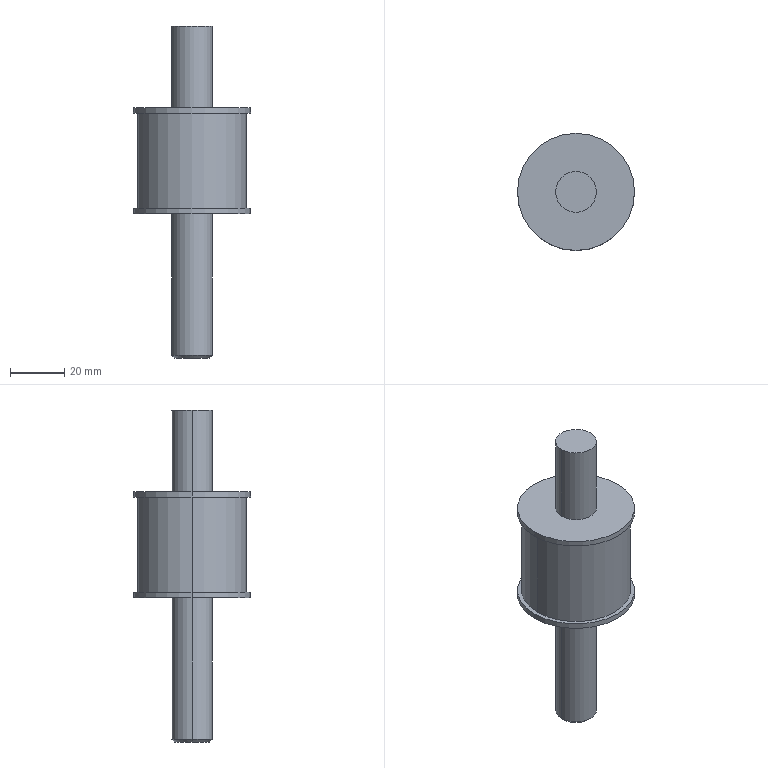Part | STEP file | Driving wheel | 1 solid | 18 faces | box 43 x 43 x 122 mm | volume 64436 mm3 | cylinder 10 | plane 6 | cone 2 | commonest cylinder face diameters 15 x4 43 x4 40 x2
STEP:
#1=CARTESIAN_POINT('',(0.,0.,0.));
#2=DIRECTION('',(0.,0.,1.));
#3=DIRECTION('',(1.,0.,0.));
#4=AXIS2_PLACEMENT_3D('',#1,#2,#3);
#5=CARTESIAN_POINT('',(-20.,0.,35.));
#6=VERTEX_POINT('',#5);
#7=CARTESIAN_POINT('',(20.,0.,35.));
#8=VERTEX_POINT('',#7);
#9=CARTESIAN_POINT('',(0.,0.,35.));
#10=DIRECTION('',(0.,0.,-1.));
#11=DIRECTION('',(-1.,0.,0.));
#12=AXIS2_PLACEMENT_3D('',#9,#10,#11);
#13=CIRCLE('',#12,20.);
#14=CARTESIAN_POINT('',(0.,0.,35.));
#15=DIRECTION('',(0.,0.,-1.));
#16=DIRECTION('',(-1.,0.,0.));
#17=AXIS2_PLACEMENT_3D('',#14,#15,#16);
#18=CYLINDRICAL_SURFACE('',#17,20.);
#19=CARTESIAN_POINT('',(0.,0.));
#20=DIRECTION('',(1.,0.));
#21=VECTOR('',#20,1.);
#22=LINE('',#19,#21);
#23=(GEOMETRIC_REPRESENTATION_CONTEXT(2)PARAMETRIC_REPRESENTATION_CONTEXT()REPRESENTATION_CONTEXT('',''));
#24=DEFINITIONAL_REPRESENTATION('',(#22),#23);
#25=PCURVE('',#18,#24);
#26=CARTESIAN_POINT('',(0.,0.,35.));
#27=DIRECTION('',(0.,0.,1.));
#28=DIRECTION('',(1.,0.,0.));
#29=AXIS2_PLACEMENT_3D('',#26,#27,#28);
#30=PLANE('',#29);
#31=CARTESIAN_POINT('',(-20.,0.));
#32=CARTESIAN_POINT('',(-20.,34.641));
#33=CARTESIAN_POINT('',(10.,17.321));
#34=CARTESIAN_POINT('',(40.,0.));
#35=CARTESIAN_POINT('',(10.,-17.321));
#36=CARTESIAN_POINT('',(-20.,-34.641));
#37=CARTESIAN_POINT('',(-20.,0.));
#38=(BOUNDED_CURVE()B_SPLINE_CURVE(2,(#31,#32,#33,#34,#35,#36,#37),.UNSPECIFIED.,.T.,.F.)B_SPLINE_CURVE_WITH_KNOTS((1,2,2,2,2,1),(-2.094,0.,2.094,4.189,6.283,8.378),.UNSPECIFIED.)CURVE()GEOMETRIC_REPRESENTATION_ITEM()RATIONAL_B_SPLINE_CURVE((1.,0.5,1.,0.5,1.,0.5,1.))REPRESENTATION_ITEM(''));
#39=(GEOMETRIC_REPRESENTATION_CONTEXT(2)PARAMETRIC_REPRESENTATION_CONTEXT()REPRESENTATION_CONTEXT('',''));
#40=DEFINITIONAL_REPRESENTATION('',(#38),#39);
#41=PCURVE('',#30,#40);
#42=SURFACE_CURVE('',#13,(#25,#41),.PCURVE_S1.);
#43=EDGE_CURVE('',#6,#8,#42,.T.);
#44=ORIENTED_EDGE('',*,*,#43,.T.);
#45=CARTESIAN_POINT('',(20.,0.,0.));
#46=VERTEX_POINT('',#45);
#47=CARTESIAN_POINT('',(20.,0.,35.));
#48=DIRECTION('',(0.,0.,-1.));
#49=VECTOR('',#48,1.);
#50=LINE('',#47,#49);
#51=CARTESIAN_POINT('',(3.142,0.));
#52=DIRECTION('',(0.,1.));
#53=VECTOR('',#52,1.);
#54=LINE('',#51,#53);
#55=(GEOMETRIC_REPRESENTATION_CONTEXT(2)PARAMETRIC_REPRESENTATION_CONTEXT()REPRESENTATION_CONTEXT('',''));
#56=DEFINITIONAL_REPRESENTATION('',(#54),#55);
#57=PCURVE('',#18,#56);
#58=CARTESIAN_POINT('',(0.,0.,35.));
#59=DIRECTION('',(0.,0.,-1.));
#60=DIRECTION('',(-1.,0.,0.));
#61=AXIS2_PLACEMENT_3D('',#58,#59,#60);
#62=CYLINDRICAL_SURFACE('',#61,20.);
#63=CARTESIAN_POINT('',(3.142,0.));
#64=DIRECTION('',(0.,1.));
#65=VECTOR('',#64,1.);
#66=LINE('',#63,#65);
#67=(GEOMETRIC_REPRESENTATION_CONTEXT(2)PARAMETRIC_REPRESENTATION_CONTEXT()REPRESENTATION_CONTEXT('',''));
#68=DEFINITIONAL_REPRESENTATION('',(#66),#67);
#69=PCURVE('',#62,#68);
#70=SURFACE_CURVE('',#50,(#57,#69),.PCURVE_S1.);
#71=EDGE_CURVE('',#8,#46,#70,.T.);
#72=ORIENTED_EDGE('',*,*,#71,.T.);
#73=CARTESIAN_POINT('',(-20.,0.,0.));
#74=VERTEX_POINT('',#73);
#75=CARTESIAN_POINT('',(0.,0.,0.));
#76=DIRECTION('',(0.,0.,1.));
#77=DIRECTION('',(-1.,0.,0.));
#78=AXIS2_PLACEMENT_3D('',#75,#76,#77);
#79=CIRCLE('',#78,20.);
#80=CARTESIAN_POINT('',(6.283,35.));
#81=DIRECTION('',(-1.,0.));
#82=VECTOR('',#81,1.);
#83=LINE('',#80,#82);
#84=(GEOMETRIC_REPRESENTATION_CONTEXT(2)PARAMETRIC_REPRESENTATION_CONTEXT()REPRESENTATION_CONTEXT('',''));
#85=DEFINITIONAL_REPRESENTATION('',(#83),#84);
#86=PCURVE('',#18,#85);
#87=CARTESIAN_POINT('',(0.,0.,0.));
#88=DIRECTION('',(0.,0.,-1.));
#89=DIRECTION('',(-1.,0.,0.));
#90=AXIS2_PLACEMENT_3D('',#87,#88,#89);
#91=PLANE('',#90);
#92=CARTESIAN_POINT('',(20.,0.));
#93=CARTESIAN_POINT('',(20.,-34.641));
#94=CARTESIAN_POINT('',(-10.,-17.321));
#95=CARTESIAN_POINT('',(-40.,0.));
#96=CARTESIAN_POINT('',(-10.,17.321));
#97=CARTESIAN_POINT('',(20.,34.641));
#98=CARTESIAN_POINT('',(20.,0.));
#99=(BOUNDED_CURVE()B_SPLINE_CURVE(2,(#92,#93,#94,#95,#96,#97,#98),.UNSPECIFIED.,.T.,.F.)B_SPLINE_CURVE_WITH_KNOTS((1,2,2,2,2,1),(-2.094,0.,2.094,4.189,6.283,8.378),.UNSPECIFIED.)CURVE()GEOMETRIC_REPRESENTATION_ITEM()RATIONAL_B_SPLINE_CURVE((1.,0.5,1.,0.5,1.,0.5,1.))REPRESENTATION_ITEM(''));
#100=(GEOMETRIC_REPRESENTATION_CONTEXT(2)PARAMETRIC_REPRESENTATION_CONTEXT()REPRESENTATION_CONTEXT('',''));
#101=DEFINITIONAL_REPRESENTATION('',(#99),#100);
#102=PCURVE('',#91,#101);
#103=SURFACE_CURVE('',#79,(#86,#102),.PCURVE_S1.);
#104=EDGE_CURVE('',#46,#74,#103,.T.);
#105=ORIENTED_EDGE('',*,*,#104,.T.);
#106=CARTESIAN_POINT('',(-20.,0.,35.));
#107=DIRECTION('',(0.,0.,-1.));
#108=VECTOR('',#107,1.);
#109=LINE('',#106,#108);
#110=CARTESIAN_POINT('',(0.,0.));
#111=DIRECTION('',(0.,1.));
#112=VECTOR('',#111,1.);
#113=LINE('',#110,#112);
#114=(GEOMETRIC_REPRESENTATION_CONTEXT(2)PARAMETRIC_REPRESENTATION_CONTEXT()REPRESENTATION_CONTEXT('',''));
#115=DEFINITIONAL_REPRESENTATION('',(#113),#114);
#116=PCURVE('',#18,#115);
#117=CARTESIAN_POINT('',(6.283,0.));
#118=DIRECTION('',(0.,1.));
#119=VECTOR('',#118,1.);
#120=LINE('',#117,#119);
#121=(GEOMETRIC_REPRESENTATION_CONTEXT(2)PARAMETRIC_REPRESENTATION_CONTEXT()REPRESENTATION_CONTEXT('',''));
#122=DEFINITIONAL_REPRESENTATION('',(#120),#121);
#123=PCURVE('',#62,#122);
#124=SURFACE_CURVE('',#109,(#116,#123),.PCURVE_S1.);
#125=EDGE_CURVE('',#6,#74,#124,.T.);
#126=ORIENTED_EDGE('',*,*,#125,.F.);
#127=EDGE_LOOP('',(#44,#72,#105,#126));
#128=FACE_BOUND('',#127,.T.);
#129=ADVANCED_FACE('',(#128),#18,.T.);
#130=CARTESIAN_POINT('',(21.5,0.,-2.));
#131=VERTEX_POINT('',#130);
#132=CARTESIAN_POINT('',(-21.5,0.,-2.));
#133=VERTEX_POINT('',#132);
#134=CARTESIAN_POINT('',(0.,0.,-2.));
#135=DIRECTION('',(0.,0.,1.));
#136=DIRECTION('',(1.,0.,0.));
#137=AXIS2_PLACEMENT_3D('',#134,#135,#136);
#138=CIRCLE('',#137,21.5);
#139=CARTESIAN_POINT('',(0.,0.,-2.));
#140=DIRECTION('',(0.,0.,1.));
#141=DIRECTION('',(1.,0.,0.));
#142=AXIS2_PLACEMENT_3D('',#139,#140,#141);
#143=CYLINDRICAL_SURFACE('',#142,21.5);
#144=CARTESIAN_POINT('',(0.,0.));
#145=DIRECTION('',(1.,0.));
#146=VECTOR('',#145,1.);
#147=LINE('',#144,#146);
#148=(GEOMETRIC_REPRESENTATION_CONTEXT(2)PARAMETRIC_REPRESENTATION_CONTEXT()REPRESENTATION_CONTEXT('',''));
#149=DEFINITIONAL_REPRESENTATION('',(#147),#148);
#150=PCURVE('',#143,#149);
#151=CARTESIAN_POINT('',(0.,0.,-2.));
#152=DIRECTION('',(0.,0.,-1.));
#153=DIRECTION('',(-1.,0.,0.));
#154=AXIS2_PLACEMENT_3D('',#151,#152,#153);
#155=PLANE('',#154);
#156=CARTESIAN_POINT('',(-21.5,0.));
#157=CARTESIAN_POINT('',(-21.5,37.239));
#158=CARTESIAN_POINT('',(10.75,18.62));
#159=CARTESIAN_POINT('',(43.,0.));
#160=CARTESIAN_POINT('',(10.75,-18.62));
#161=CARTESIAN_POINT('',(-21.5,-37.239));
#162=CARTESIAN_POINT('',(-21.5,0.));
#163=(BOUNDED_CURVE()B_SPLINE_CURVE(2,(#156,#157,#158,#159,#160,#161,#162),.UNSPECIFIED.,.T.,.F.)B_SPLINE_CURVE_WITH_KNOTS((1,2,2,2,2,1),(-2.094,0.,2.094,4.189,6.283,8.378),.UNSPECIFIED.)CURVE()GEOMETRIC_REPRESENTATION_ITEM()RATIONAL_B_SPLINE_CURVE((1.,0.5,1.,0.5,1.,0.5,1.))REPRESENTATION_ITEM(''));
#164=(GEOMETRIC_REPRESENTATION_CONTEXT(2)PARAMETRIC_REPRESENTATION_CONTEXT()REPRESENTATION_CONTEXT('',''));
#165=DEFINITIONAL_REPRESENTATION('',(#163),#164);
#166=PCURVE('',#155,#165);
#167=SURFACE_CURVE('',#138,(#150,#166),.PCURVE_S1.);
#168=EDGE_CURVE('',#131,#133,#167,.T.);
#169=ORIENTED_EDGE('',*,*,#168,.T.);
#170=CARTESIAN_POINT('',(-21.5,0.,0.));
#171=VERTEX_POINT('',#170);
#172=CARTESIAN_POINT('',(-21.5,0.,-2.));
#173=DIRECTION('',(0.,0.,1.));
#174=VECTOR('',#173,1.);
#175=LINE('',#172,#174);
#176=CARTESIAN_POINT('',(3.142,0.));
#177=DIRECTION('',(0.,1.));
#178=VECTOR('',#177,1.);
#179=LINE('',#176,#178);
#180=(GEOMETRIC_REPRESENTATION_CONTEXT(2)PARAMETRIC_REPRESENTATION_CONTEXT()REPRESENTATION_CONTEXT('',''));
#181=DEFINITIONAL_REPRESENTATION('',(#179),#180);
#182=PCURVE('',#143,#181);
#183=CARTESIAN_POINT('',(0.,0.,-2.));
#184=DIRECTION('',(0.,0.,1.));
#185=DIRECTION('',(1.,0.,0.));
#186=AXIS2_PLACEMENT_3D('',#183,#184,#185);
#187=CYLINDRICAL_SURFACE('',#186,21.5);
#188=CARTESIAN_POINT('',(3.142,0.));
#189=DIRECTION('',(0.,1.));
#190=VECTOR('',#189,1.);
#191=LINE('',#188,#190);
#192=(GEOMETRIC_REPRESENTATION_CONTEXT(2)PARAMETRIC_REPRESENTATION_CONTEXT()REPRESENTATION_CONTEXT('',''));
#193=DEFINITIONAL_REPRESENTATION('',(#191),#192);
#194=PCURVE('',#187,#193);
#195=SURFACE_CURVE('',#175,(#182,#194),.PCURVE_S1.);
#196=EDGE_CURVE('',#133,#171,#195,.T.);
#197=ORIENTED_EDGE('',*,*,#196,.T.);
#198=CARTESIAN_POINT('',(21.5,0.,0.));
#199=VERTEX_POINT('',#198);
#200=CARTESIAN_POINT('',(0.,0.,0.));
#201=DIRECTION('',(0.,0.,-1.));
#202=DIRECTION('',(1.,0.,0.));
#203=AXIS2_PLACEMENT_3D('',#200,#201,#202);
#204=CIRCLE('',#203,21.5);
#205=CARTESIAN_POINT('',(6.283,2.));
#206=DIRECTION('',(-1.,0.));
#207=VECTOR('',#206,1.);
#208=LINE('',#205,#207);
#209=(GEOMETRIC_REPRESENTATION_CONTEXT(2)PARAMETRIC_REPRESENTATION_CONTEXT()REPRESENTATION_CONTEXT('',''));
#210=DEFINITIONAL_REPRESENTATION('',(#208),#209);
#211=PCURVE('',#143,#210);
#212=CARTESIAN_POINT('',(0.,0.));
#213=DIRECTION('',(-1.,0.));
#214=AXIS2_PLACEMENT_2D('',#212,#213);
#215=CIRCLE('',#214,21.5);
#216=(GEOMETRIC_REPRESENTATION_CONTEXT(2)PARAMETRIC_REPRESENTATION_CONTEXT()REPRESENTATION_CONTEXT('',''));
#217=DEFINITIONAL_REPRESENTATION('',(#215),#216);
#218=PCURVE('',#91,#217);
#219=SURFACE_CURVE('',#204,(#211,#218),.PCURVE_S1.);
#220=EDGE_CURVE('',#171,#199,#219,.T.);
#221=ORIENTED_EDGE('',*,*,#220,.T.);
#222=CARTESIAN_POINT('',(21.5,0.,-2.));
#223=DIRECTION('',(0.,0.,1.));
#224=VECTOR('',#223,1.);
#225=LINE('',#222,#224);
#226=CARTESIAN_POINT('',(0.,0.));
#227=DIRECTION('',(0.,1.));
#228=VECTOR('',#227,1.);
#229=LINE('',#226,#228);
#230=(GEOMETRIC_REPRESENTATION_CONTEXT(2)PARAMETRIC_REPRESENTATION_CONTEXT()REPRESENTATION_CONTEXT('',''));
#231=DEFINITIONAL_REPRESENTATION('',(#229),#230);
#232=PCURVE('',#143,#231);
#233=CARTESIAN_POINT('',(6.283,0.));
#234=DIRECTION('',(0.,1.));
#235=VECTOR('',#234,1.);
#236=LINE('',#233,#235);
#237=(GEOMETRIC_REPRESENTATION_CONTEXT(2)PARAMETRIC_REPRESENTATION_CONTEXT()REPRESENTATION_CONTEXT('',''));
#238=DEFINITIONAL_REPRESENTATION('',(#236),#237);
#239=PCURVE('',#187,#238);
#240=SURFACE_CURVE('',#225,(#232,#239),.PCURVE_S1.);
#241=EDGE_CURVE('',#131,#199,#240,.T.);
#242=ORIENTED_EDGE('',*,*,#241,.F.);
#243=EDGE_LOOP('',(#169,#197,#221,#242));
#244=FACE_BOUND('',#243,.T.);
#245=ADVANCED_FACE('',(#244),#143,.T.);
#246=CARTESIAN_POINT('',(-21.5,0.,37.));
#247=VERTEX_POINT('',#246);
#248=CARTESIAN_POINT('',(21.5,0.,37.));
#249=VERTEX_POINT('',#248);
#250=CARTESIAN_POINT('',(0.,0.,37.));
#251=DIRECTION('',(0.,0.,-1.));
#252=DIRECTION('',(-1.,0.,0.));
#253=AXIS2_PLACEMENT_3D('',#250,#251,#252);
#254=CIRCLE('',#253,21.5);
#255=CARTESIAN_POINT('',(0.,0.,37.));
#256=DIRECTION('',(0.,0.,-1.));
#257=DIRECTION('',(-1.,0.,0.));
#258=AXIS2_PLACEMENT_3D('',#255,#256,#257);
#259=CYLINDRICAL_SURFACE('',#258,21.5);
#260=CARTESIAN_POINT('',(0.,0.));
#261=DIRECTION('',(1.,0.));
#262=VECTOR('',#261,1.);
#263=LINE('',#260,#262);
#264=(GEOMETRIC_REPRESENTATION_CONTEXT(2)PARAMETRIC_REPRESENTATION_CONTEXT()REPRESENTATION_CONTEXT('',''));
#265=DEFINITIONAL_REPRESENTATION('',(#263),#264);
#266=PCURVE('',#259,#265);
#267=CARTESIAN_POINT('',(0.,0.,37.));
#268=DIRECTION('',(0.,0.,1.));
#269=DIRECTION('',(1.,0.,0.));
#270=AXIS2_PLACEMENT_3D('',#267,#268,#269);
#271=PLANE('',#270);
#272=CARTESIAN_POINT('',(-21.5,0.));
#273=CARTESIAN_POINT('',(-21.5,37.239));
#274=CARTESIAN_POINT('',(10.75,18.62));
#275=CARTESIAN_POINT('',(43.,0.));
#276=CARTESIAN_POINT('',(10.75,-18.62));
#277=CARTESIAN_POINT('',(-21.5,-37.239));
#278=CARTESIAN_POINT('',(-21.5,0.));
#279=(BOUNDED_CURVE()B_SPLINE_CURVE(2,(#272,#273,#274,#275,#276,#277,#278),.UNSPECIFIED.,.T.,.F.)B_SPLINE_CURVE_WITH_KNOTS((1,2,2,2,2,1),(-2.094,0.,2.094,4.189,6.283,8.378),.UNSPECIFIED.)CURVE()GEOMETRIC_REPRESENTATION_ITEM()RATIONAL_B_SPLINE_CURVE((1.,0.5,1.,0.5,1.,0.5,1.))REPRESENTATION_ITEM(''));
#280=(GEOMETRIC_REPRESENTATION_CONTEXT(2)PARAMETRIC_REPRESENTATION_CONTEXT()REPRESENTATION_CONTEXT('',''));
#281=DEFINITIONAL_REPRESENTATION('',(#279),#280);
#282=PCURVE('',#271,#281);
#283=SURFACE_CURVE('',#254,(#266,#282),.PCURVE_S1.);
#284=EDGE_CURVE('',#247,#249,#283,.T.);
#285=ORIENTED_EDGE('',*,*,#284,.T.);
#286=CARTESIAN_POINT('',(21.5,0.,35.));
#287=VERTEX_POINT('',#286);
#288=CARTESIAN_POINT('',(21.5,0.,37.));
#289=DIRECTION('',(0.,0.,-1.));
#290=VECTOR('',#289,1.);
#291=LINE('',#288,#290);
#292=CARTESIAN_POINT('',(3.142,0.));
#293=DIRECTION('',(0.,1.));
#294=VECTOR('',#293,1.);
#295=LINE('',#292,#294);
#296=(GEOMETRIC_REPRESENTATION_CONTEXT(2)PARAMETRIC_REPRESENTATION_CONTEXT()REPRESENTATION_CONTEXT('',''));
#297=DEFINITIONAL_REPRESENTATION('',(#295),#296);
#298=PCURVE('',#259,#297);
#299=CARTESIAN_POINT('',(0.,0.,37.));
#300=DIRECTION('',(0.,0.,-1.));
#301=DIRECTION('',(-1.,0.,0.));
#302=AXIS2_PLACEMENT_3D('',#299,#300,#301);
#303=CYLINDRICAL_SURFACE('',#302,21.5);
#304=CARTESIAN_POINT('',(3.142,0.));
#305=DIRECTION('',(0.,1.));
#306=VECTOR('',#305,1.);
#307=LINE('',#304,#306);
#308=(GEOMETRIC_REPRESENTATION_CONTEXT(2)PARAMETRIC_REPRESENTATION_CONTEXT()REPRESENTATION_CONTEXT('',''));
#309=DEFINITIONAL_REPRESENTATION('',(#307),#308);
#310=PCURVE('',#303,#309);
#311=SURFACE_CURVE('',#291,(#298,#310),.PCURVE_S1.);
#312=EDGE_CURVE('',#249,#287,#311,.T.);
#313=ORIENTED_EDGE('',*,*,#312,.T.);
#314=CARTESIAN_POINT('',(-21.5,0.,35.));
#315=VERTEX_POINT('',#314);
#316=CARTESIAN_POINT('',(0.,0.,35.));
#317=DIRECTION('',(0.,0.,1.));
#318=DIRECTION('',(-1.,0.,0.));
#319=AXIS2_PLACEMENT_3D('',#316,#317,#318);
#320=CIRCLE('',#319,21.5);
#321=CARTESIAN_POINT('',(6.283,2.));
#322=DIRECTION('',(-1.,0.));
#323=VECTOR('',#322,1.);
#324=LINE('',#321,#323);
#325=(GEOMETRIC_REPRESENTATION_CONTEXT(2)PARAMETRIC_REPRESENTATION_CONTEXT()REPRESENTATION_CONTEXT('',''));
#326=DEFINITIONAL_REPRESENTATION('',(#324),#325);
#327=PCURVE('',#259,#326);
#328=CARTESIAN_POINT('',(0.,0.));
#329=DIRECTION('',(-1.,0.));
#330=AXIS2_PLACEMENT_2D('',#328,#329);
#331=CIRCLE('',#330,21.5);
#332=(GEOMETRIC_REPRESENTATION_CONTEXT(2)PARAMETRIC_REPRESENTATION_CONTEXT()REPRESENTATION_CONTEXT('',''));
#333=DEFINITIONAL_REPRESENTATION('',(#331),#332);
#334=PCURVE('',#30,#333);
#335=SURFACE_CURVE('',#320,(#327,#334),.PCURVE_S1.);
#336=EDGE_CURVE('',#287,#315,#335,.T.);
#337=ORIENTED_EDGE('',*,*,#336,.T.);
#338=CARTESIAN_POINT('',(-21.5,0.,37.));
#339=DIRECTION('',(0.,0.,-1.));
#340=VECTOR('',#339,1.);
#341=LINE('',#338,#340);
#342=CARTESIAN_POINT('',(0.,0.));
#343=DIRECTION('',(0.,1.));
#344=VECTOR('',#343,1.);
#345=LINE('',#342,#344);
#346=(GEOMETRIC_REPRESENTATION_CONTEXT(2)PARAMETRIC_REPRESENTATION_CONTEXT()REPRESENTATION_CONTEXT('',''));
#347=DEFINITIONAL_REPRESENTATION('',(#345),#346);
#348=PCURVE('',#259,#347);
#349=CARTESIAN_POINT('',(6.283,0.));
#350=DIRECTION('',(0.,1.));
#351=VECTOR('',#350,1.);
#352=LINE('',#349,#351);
#353=(GEOMETRIC_REPRESENTATION_CONTEXT(2)PARAMETRIC_REPRESENTATION_CONTEXT()REPRESENTATION_CONTEXT('',''));
#354=DEFINITIONAL_REPRESENTATION('',(#352),#353);
#355=PCURVE('',#303,#354);
#356=SURFACE_CURVE('',#341,(#348,#355),.PCURVE_S1.);
#357=EDGE_CURVE('',#247,#315,#356,.T.);
#358=ORIENTED_EDGE('',*,*,#357,.F.);
#359=EDGE_LOOP('',(#285,#313,#337,#358));
#360=FACE_BOUND('',#359,.T.);
#361=ADVANCED_FACE('',(#360),#259,.T.);
#362=CARTESIAN_POINT('',(7.5,0.,-54.));
#363=VERTEX_POINT('',#362);
#364=CARTESIAN_POINT('',(-7.5,0.,-54.));
#365=VERTEX_POINT('',#364);
#366=CARTESIAN_POINT('',(0.,0.,-54.));
#367=DIRECTION('',(0.,0.,1.));
#368=DIRECTION('',(1.,0.,0.));
#369=AXIS2_PLACEMENT_3D('',#366,#367,#368);
#370=CIRCLE('',#369,7.5);
#371=CARTESIAN_POINT('',(0.,0.,-55.));
#372=DIRECTION('',(0.,0.,1.));
#373=DIRECTION('',(1.,0.,0.));
#374=AXIS2_PLACEMENT_3D('',#371,#372,#373);
#375=CYLINDRICAL_SURFACE('',#374,7.5);
#376=CARTESIAN_POINT('',(0.,1.));
#377=DIRECTION('',(1.,0.));
#378=VECTOR('',#377,1.);
#379=LINE('',#376,#378);
#380=(GEOMETRIC_REPRESENTATION_CONTEXT(2)PARAMETRIC_REPRESENTATION_CONTEXT()REPRESENTATION_CONTEXT('',''));
#381=DEFINITIONAL_REPRESENTATION('',(#379),#380);
#382=PCURVE('',#375,#381);
#383=CARTESIAN_POINT('',(0.,0.,-54.));
#384=DIRECTION('',(0.,0.,1.));
#385=DIRECTION('',(1.,0.,0.));
#386=AXIS2_PLACEMENT_3D('',#383,#384,#385);
#387=CONICAL_SURFACE('',#386,7.5,0.7854);
#388=CARTESIAN_POINT('',(0.,0.));
#389=DIRECTION('',(1.,0.));
#390=VECTOR('',#389,1.);
#391=LINE('',#388,#390);
#392=(GEOMETRIC_REPRESENTATION_CONTEXT(2)PARAMETRIC_REPRESENTATION_CONTEXT()REPRESENTATION_CONTEXT('',''));
#393=DEFINITIONAL_REPRESENTATION('',(#391),#392);
#394=PCURVE('',#387,#393);
#395=SURFACE_CURVE('',#370,(#382,#394),.PCURVE_S1.);
#396=EDGE_CURVE('',#363,#365,#395,.T.);
#397=ORIENTED_EDGE('',*,*,#396,.T.);
#398=CARTESIAN_POINT('',(-7.5,0.,-2.));
#399=VERTEX_POINT('',#398);
#400=CARTESIAN_POINT('',(-7.5,0.,-55.));
#401=DIRECTION('',(0.,0.,1.));
#402=VECTOR('',#401,1.);
#403=LINE('',#400,#402);
#404=CARTESIAN_POINT('',(3.142,0.));
#405=DIRECTION('',(0.,1.));
#406=VECTOR('',#405,1.);
#407=LINE('',#404,#406);
#408=(GEOMETRIC_REPRESENTATION_CONTEXT(2)PARAMETRIC_REPRESENTATION_CONTEXT()REPRESENTATION_CONTEXT('',''));
#409=DEFINITIONAL_REPRESENTATION('',(#407),#408);
#410=PCURVE('',#375,#409);
#411=CARTESIAN_POINT('',(0.,0.,-55.));
#412=DIRECTION('',(0.,0.,1.));
#413=DIRECTION('',(1.,0.,0.));
#414=AXIS2_PLACEMENT_3D('',#411,#412,#413);
#415=CYLINDRICAL_SURFACE('',#414,7.5);
#416=CARTESIAN_POINT('',(3.142,0.));
#417=DIRECTION('',(0.,1.));
#418=VECTOR('',#417,1.);
#419=LINE('',#416,#418);
#420=(GEOMETRIC_REPRESENTATION_CONTEXT(2)PARAMETRIC_REPRESENTATION_CONTEXT()REPRESENTATION_CONTEXT('',''));
#421=DEFINITIONAL_REPRESENTATION('',(#419),#420);
#422=PCURVE('',#415,#421);
#423=SURFACE_CURVE('',#403,(#410,#422),.PCURVE_S1.);
#424=EDGE_CURVE('',#365,#399,#423,.T.);
#425=ORIENTED_EDGE('',*,*,#424,.T.);
#426=CARTESIAN_POINT('',(7.5,0.,-2.));
#427=VERTEX_POINT('',#426);
#428=CARTESIAN_POINT('',(0.,0.,-2.));
#429=DIRECTION('',(0.,0.,1.));
#430=DIRECTION('',(1.,0.,0.));
#431=AXIS2_PLACEMENT_3D('',#428,#429,#430);
#432=CIRCLE('',#431,7.5);
#433=CARTESIAN_POINT('',(0.,53.));
#434=DIRECTION('',(1.,0.));
#435=VECTOR('',#434,1.);
#436=LINE('',#433,#435);
#437=(GEOMETRIC_REPRESENTATION_CONTEXT(2)PARAMETRIC_REPRESENTATION_CONTEXT()REPRESENTATION_CONTEXT('',''));
#438=DEFINITIONAL_REPRESENTATION('',(#436),#437);
#439=PCURVE('',#375,#438);
#440=CARTESIAN_POINT('',(-7.5,0.));
#441=CARTESIAN_POINT('',(-7.5,12.99));
#442=CARTESIAN_POINT('',(3.75,6.495));
#443=CARTESIAN_POINT('',(15.,0.));
#444=CARTESIAN_POINT('',(3.75,-6.495));
#445=CARTESIAN_POINT('',(-7.5,-12.99));
#446=CARTESIAN_POINT('',(-7.5,0.));
#447=(BOUNDED_CURVE()B_SPLINE_CURVE(2,(#440,#441,#442,#443,#444,#445,#446),.UNSPECIFIED.,.T.,.F.)B_SPLINE_CURVE_WITH_KNOTS((1,2,2,2,2,1),(-2.094,0.,2.094,4.189,6.283,8.378),.UNSPECIFIED.)CURVE()GEOMETRIC_REPRESENTATION_ITEM()RATIONAL_B_SPLINE_CURVE((1.,0.5,1.,0.5,1.,0.5,1.))REPRESENTATION_ITEM(''));
#448=(GEOMETRIC_REPRESENTATION_CONTEXT(2)PARAMETRIC_REPRESENTATION_CONTEXT()REPRESENTATION_CONTEXT('',''));
#449=DEFINITIONAL_REPRESENTATION('',(#447),#448);
#450=PCURVE('',#155,#449);
#451=SURFACE_CURVE('',#432,(#439,#450),.PCURVE_S1.);
#452=EDGE_CURVE('',#427,#399,#451,.T.);
#453=ORIENTED_EDGE('',*,*,#452,.F.);
#454=CARTESIAN_POINT('',(7.5,0.,-55.));
#455=DIRECTION('',(0.,0.,1.));
#456=VECTOR('',#455,1.);
#457=LINE('',#454,#456);
#458=CARTESIAN_POINT('',(0.,0.));
#459=DIRECTION('',(0.,1.));
#460=VECTOR('',#459,1.);
#461=LINE('',#458,#460);
#462=(GEOMETRIC_REPRESENTATION_CONTEXT(2)PARAMETRIC_REPRESENTATION_CONTEXT()REPRESENTATION_CONTEXT('',''));
#463=DEFINITIONAL_REPRESENTATION('',(#461),#462);
#464=PCURVE('',#375,#463);
#465=CARTESIAN_POINT('',(6.283,0.));
#466=DIRECTION('',(0.,1.));
#467=VECTOR('',#466,1.);
#468=LINE('',#465,#467);
#469=(GEOMETRIC_REPRESENTATION_CONTEXT(2)PARAMETRIC_REPRESENTATION_CONTEXT()REPRESENTATION_CONTEXT('',''));
#470=DEFINITIONAL_REPRESENTATION('',(#468),#469);
#471=PCURVE('',#415,#470);
#472=SURFACE_CURVE('',#457,(#464,#471),.PCURVE_S1.);
#473=EDGE_CURVE('',#363,#427,#472,.T.);
#474=ORIENTED_EDGE('',*,*,#473,.F.);
#475=EDGE_LOOP('',(#397,#425,#453,#474));
#476=FACE_BOUND('',#475,.T.);
#477=ADVANCED_FACE('',(#476),#375,.T.);
#478=CARTESIAN_POINT('',(-7.5,0.,67.));
#479=VERTEX_POINT('',#478);
#480=CARTESIAN_POINT('',(7.5,0.,67.));
#481=VERTEX_POINT('',#480);
#482=CARTESIAN_POINT('',(0.,0.,67.));
#483=DIRECTION('',(0.,0.,-1.));
#484=DIRECTION('',(-1.,0.,0.));
#485=AXIS2_PLACEMENT_3D('',#482,#483,#484);
#486=CIRCLE('',#485,7.5);
#487=CARTESIAN_POINT('',(0.,0.,67.));
#488=DIRECTION('',(0.,0.,-1.));
#489=DIRECTION('',(-1.,0.,0.));
#490=AXIS2_PLACEMENT_3D('',#487,#488,#489);
#491=CYLINDRICAL_SURFACE('',#490,7.5);
#492=CARTESIAN_POINT('',(0.,0.));
#493=DIRECTION('',(1.,0.));
#494=VECTOR('',#493,1.);
#495=LINE('',#492,#494);
#496=(GEOMETRIC_REPRESENTATION_CONTEXT(2)PARAMETRIC_REPRESENTATION_CONTEXT()REPRESENTATION_CONTEXT('',''));
#497=DEFINITIONAL_REPRESENTATION('',(#495),#496);
#498=PCURVE('',#491,#497);
#499=CARTESIAN_POINT('',(0.,0.,67.));
#500=DIRECTION('',(0.,0.,1.));
#501=DIRECTION('',(1.,0.,0.));
#502=AXIS2_PLACEMENT_3D('',#499,#500,#501);
#503=PLANE('',#502);
#504=CARTESIAN_POINT('',(-7.5,0.));
#505=CARTESIAN_POINT('',(-7.5,12.99));
#506=CARTESIAN_POINT('',(3.75,6.495));
#507=CARTESIAN_POINT('',(15.,0.));
#508=CARTESIAN_POINT('',(3.75,-6.495));
#509=CARTESIAN_POINT('',(-7.5,-12.99));
#510=CARTESIAN_POINT('',(-7.5,0.));
#511=(BOUNDED_CURVE()B_SPLINE_CURVE(2,(#504,#505,#506,#507,#508,#509,#510),.UNSPECIFIED.,.T.,.F.)B_SPLINE_CURVE_WITH_KNOTS((1,2,2,2,2,1),(-2.094,0.,2.094,4.189,6.283,8.378),.UNSPECIFIED.)CURVE()GEOMETRIC_REPRESENTATION_ITEM()RATIONAL_B_SPLINE_CURVE((1.,0.5,1.,0.5,1.,0.5,1.))REPRESENTATION_ITEM(''));
#512=(GEOMETRIC_REPRESENTATION_CONTEXT(2)PARAMETRIC_REPRESENTATION_CONTEXT()REPRESENTATION_CONTEXT('',''));
#513=DEFINITIONAL_REPRESENTATION('',(#511),#512);
#514=PCURVE('',#503,#513);
#515=SURFACE_CURVE('',#486,(#498,#514),.PCURVE_S1.);
#516=EDGE_CURVE('',#479,#481,#515,.T.);
#517=ORIENTED_EDGE('',*,*,#516,.T.);
#518=CARTESIAN_POINT('',(7.5,0.,37.));
#519=VERTEX_POINT('',#518);
#520=CARTESIAN_POINT('',(7.5,0.,67.));
#521=DIRECTION('',(0.,0.,-1.));
#522=VECTOR('',#521,1.);
#523=LINE('',#520,#522);
#524=CARTESIAN_POINT('',(3.142,0.));
#525=DIRECTION('',(0.,1.));
#526=VECTOR('',#525,1.);
#527=LINE('',#524,#526);
#528=(GEOMETRIC_REPRESENTATION_CONTEXT(2)PARAMETRIC_REPRESENTATION_CONTEXT()REPRESENTATION_CONTEXT('',''));
#529=DEFINITIONAL_REPRESENTATION('',(#527),#528);
#530=PCURVE('',#491,#529);
#531=CARTESIAN_POINT('',(0.,0.,67.));
#532=DIRECTION('',(0.,0.,-1.));
#533=DIRECTION('',(-1.,0.,0.));
#534=AXIS2_PLACEMENT_3D('',#531,#532,#533);
#535=CYLINDRICAL_SURFACE('',#534,7.5);
#536=CARTESIAN_POINT('',(3.142,0.));
#537=DIRECTION('',(0.,1.));
#538=VECTOR('',#537,1.);
#539=LINE('',#536,#538);
#540=(GEOMETRIC_REPRESENTATION_CONTEXT(2)PARAMETRIC_REPRESENTATION_CONTEXT()REPRESENTATION_CONTEXT('',''));
#541=DEFINITIONAL_REPRESENTATION('',(#539),#540);
#542=PCURVE('',#535,#541);
#543=SURFACE_CURVE('',#523,(#530,#542),.PCURVE_S1.);
#544=EDGE_CURVE('',#481,#519,#543,.T.);
#545=ORIENTED_EDGE('',*,*,#544,.T.);
#546=CARTESIAN_POINT('',(-7.5,0.,37.));
#547=VERTEX_POINT('',#546);
#548=CARTESIAN_POINT('',(0.,0.,37.));
#549=DIRECTION('',(0.,0.,-1.));
#550=DIRECTION('',(-1.,0.,0.));
#551=AXIS2_PLACEMENT_3D('',#548,#549,#550);
#552=CIRCLE('',#551,7.5);
#553=CARTESIAN_POINT('',(0.,30.));
#554=DIRECTION('',(1.,0.));
#555=VECTOR('',#554,1.);
#556=LINE('',#553,#555);
#557=(GEOMETRIC_REPRESENTATION_CONTEXT(2)PARAMETRIC_REPRESENTATION_CONTEXT()REPRESENTATION_CONTEXT('',''));
#558=DEFINITIONAL_REPRESENTATION('',(#556),#557);
#559=PCURVE('',#491,#558);
#560=CARTESIAN_POINT('',(-7.5,0.));
#561=CARTESIAN_POINT('',(-7.5,12.99));
#562=CARTESIAN_POINT('',(3.75,6.495));
#563=CARTESIAN_POINT('',(15.,0.));
#564=CARTESIAN_POINT('',(3.75,-6.495));
#565=CARTESIAN_POINT('',(-7.5,-12.99));
#566=CARTESIAN_POINT('',(-7.5,0.));
#567=(BOUNDED_CURVE()B_SPLINE_CURVE(2,(#560,#561,#562,#563,#564,#565,#566),.UNSPECIFIED.,.T.,.F.)B_SPLINE_CURVE_WITH_KNOTS((1,2,2,2,2,1),(-2.094,0.,2.094,4.189,6.283,8.378),.UNSPECIFIED.)CURVE()GEOMETRIC_REPRESENTATION_ITEM()RATIONAL_B_SPLINE_CURVE((1.,0.5,1.,0.5,1.,0.5,1.))REPRESENTATION_ITEM(''));
#568=(GEOMETRIC_REPRESENTATION_CONTEXT(2)PARAMETRIC_REPRESENTATION_CONTEXT()REPRESENTATION_CONTEXT('',''));
#569=DEFINITIONAL_REPRESENTATION('',(#567),#568);
#570=PCURVE('',#271,#569);
#571=SURFACE_CURVE('',#552,(#559,#570),.PCURVE_S1.);
#572=EDGE_CURVE('',#547,#519,#571,.T.);
#573=ORIENTED_EDGE('',*,*,#572,.F.);
#574=CARTESIAN_POINT('',(-7.5,0.,67.));
#575=DIRECTION('',(0.,0.,-1.));
#576=VECTOR('',#575,1.);
#577=LINE('',#574,#576);
#578=CARTESIAN_POINT('',(0.,0.));
#579=DIRECTION('',(0.,1.));
#580=VECTOR('',#579,1.);
#581=LINE('',#578,#580);
#582=(GEOMETRIC_REPRESENTATION_CONTEXT(2)PARAMETRIC_REPRESENTATION_CONTEXT()REPRESENTATION_CONTEXT('',''));
#583=DEFINITIONAL_REPRESENTATION('',(#581),#582);
#584=PCURVE('',#491,#583);
#585=CARTESIAN_POINT('',(6.283,0.));
#586=DIRECTION('',(0.,1.));
#587=VECTOR('',#586,1.);
#588=LINE('',#585,#587);
#589=(GEOMETRIC_REPRESENTATION_CONTEXT(2)PARAMETRIC_REPRESENTATION_CONTEXT()REPRESENTATION_CONTEXT('',''));
#590=DEFINITIONAL_REPRESENTATION('',(#588),#589);
#591=PCURVE('',#535,#590);
#592=SURFACE_CURVE('',#577,(#584,#591),.PCURVE_S1.);
#593=EDGE_CURVE('',#479,#547,#592,.T.);
#594=ORIENTED_EDGE('',*,*,#593,.F.);
#595=EDGE_LOOP('',(#517,#545,#573,#594));
#596=FACE_BOUND('',#595,.T.);
#597=ADVANCED_FACE('',(#596),#491,.T.);
#598=CARTESIAN_POINT('',(6.5,0.,-55.));
#599=VERTEX_POINT('',#598);
#600=CARTESIAN_POINT('',(-6.5,0.,-55.));
#601=VERTEX_POINT('',#600);
#602=CARTESIAN_POINT('',(0.,0.,-55.));
#603=DIRECTION('',(0.,0.,1.));
#604=DIRECTION('',(1.,0.,0.));
#605=AXIS2_PLACEMENT_3D('',#602,#603,#604);
#606=CIRCLE('',#605,6.5);
#607=CARTESIAN_POINT('',(0.,-1.));
#608=DIRECTION('',(1.,0.));
#609=VECTOR('',#608,1.);
#610=LINE('',#607,#609);
#611=(GEOMETRIC_REPRESENTATION_CONTEXT(2)PARAMETRIC_REPRESENTATION_CONTEXT()REPRESENTATION_CONTEXT('',''));
#612=DEFINITIONAL_REPRESENTATION('',(#610),#611);
#613=PCURVE('',#387,#612);
#614=CARTESIAN_POINT('',(0.,0.,-55.));
#615=DIRECTION('',(0.,0.,-1.));
#616=DIRECTION('',(-1.,0.,0.));
#617=AXIS2_PLACEMENT_3D('',#614,#615,#616);
#618=PLANE('',#617);
#619=CARTESIAN_POINT('',(-6.5,0.));
#620=CARTESIAN_POINT('',(-6.5,11.258));
#621=CARTESIAN_POINT('',(3.25,5.629));
#622=CARTESIAN_POINT('',(13.,0.));
#623=CARTESIAN_POINT('',(3.25,-5.629));
#624=CARTESIAN_POINT('',(-6.5,-11.258));
#625=CARTESIAN_POINT('',(-6.5,0.));
#626=(BOUNDED_CURVE()B_SPLINE_CURVE(2,(#619,#620,#621,#622,#623,#624,#625),.UNSPECIFIED.,.T.,.F.)B_SPLINE_CURVE_WITH_KNOTS((1,2,2,2,2,1),(-2.094,0.,2.094,4.189,6.283,8.378),.UNSPECIFIED.)CURVE()GEOMETRIC_REPRESENTATION_ITEM()RATIONAL_B_SPLINE_CURVE((1.,0.5,1.,0.5,1.,0.5,1.))REPRESENTATION_ITEM(''));
#627=(GEOMETRIC_REPRESENTATION_CONTEXT(2)PARAMETRIC_REPRESENTATION_CONTEXT()REPRESENTATION_CONTEXT('',''));
#628=DEFINITIONAL_REPRESENTATION('',(#626),#627);
#629=PCURVE('',#618,#628);
#630=SURFACE_CURVE('',#606,(#613,#629),.PCURVE_S1.);
#631=EDGE_CURVE('',#599,#601,#630,.T.);
#632=ORIENTED_EDGE('',*,*,#631,.T.);
#633=CARTESIAN_POINT('',(-7.5,0.,-54.));
#634=DIRECTION('',(-0.7071,0.,0.7071));
#635=VECTOR('',#634,1.);
#636=LINE('',#633,#635);
#637=CARTESIAN_POINT('',(3.142,0.));
#638=DIRECTION('',(0.,1.));
#639=VECTOR('',#638,1.);
#640=LINE('',#637,#639);
#641=(GEOMETRIC_REPRESENTATION_CONTEXT(2)PARAMETRIC_REPRESENTATION_CONTEXT()REPRESENTATION_CONTEXT('',''));
#642=DEFINITIONAL_REPRESENTATION('',(#640),#641);
#643=PCURVE('',#387,#642);
#644=CARTESIAN_POINT('',(0.,0.,-54.));
#645=DIRECTION('',(0.,0.,1.));
#646=DIRECTION('',(1.,0.,0.));
#647=AXIS2_PLACEMENT_3D('',#644,#645,#646);
#648=CONICAL_SURFACE('',#647,7.5,0.7854);
#649=CARTESIAN_POINT('',(3.142,0.));
#650=DIRECTION('',(0.,1.));
#651=VECTOR('',#650,1.);
#652=LINE('',#649,#651);
#653=(GEOMETRIC_REPRESENTATION_CONTEXT(2)PARAMETRIC_REPRESENTATION_CONTEXT()REPRESENTATION_CONTEXT('',''));
#654=DEFINITIONAL_REPRESENTATION('',(#652),#653);
#655=PCURVE('',#648,#654);
#656=SURFACE_CURVE('',#636,(#643,#655),.PCURVE_S1.);
#657=EDGE_CURVE('',#601,#365,#656,.T.);
#658=ORIENTED_EDGE('',*,*,#657,.T.);
#659=ORIENTED_EDGE('',*,*,#396,.F.);
#660=CARTESIAN_POINT('',(7.5,0.,-54.));
#661=DIRECTION('',(0.7071,0.,0.7071));
#662=VECTOR('',#661,1.);
#663=LINE('',#660,#662);
#664=CARTESIAN_POINT('',(0.,0.));
#665=DIRECTION('',(0.,1.));
#666=VECTOR('',#665,1.);
#667=LINE('',#664,#666);
#668=(GEOMETRIC_REPRESENTATION_CONTEXT(2)PARAMETRIC_REPRESENTATION_CONTEXT()REPRESENTATION_CONTEXT('',''));
#669=DEFINITIONAL_REPRESENTATION('',(#667),#668);
#670=PCURVE('',#387,#669);
#671=CARTESIAN_POINT('',(6.283,0.));
#672=DIRECTION('',(0.,1.));
#673=VECTOR('',#672,1.);
#674=LINE('',#671,#673);
#675=(GEOMETRIC_REPRESENTATION_CONTEXT(2)PARAMETRIC_REPRESENTATION_CONTEXT()REPRESENTATION_CONTEXT('',''));
#676=DEFINITIONAL_REPRESENTATION('',(#674),#675);
#677=PCURVE('',#648,#676);
#678=SURFACE_CURVE('',#663,(#670,#677),.PCURVE_S1.);
#679=EDGE_CURVE('',#599,#363,#678,.T.);
#680=ORIENTED_EDGE('',*,*,#679,.F.);
#681=EDGE_LOOP('',(#632,#658,#659,#680));
#682=FACE_BOUND('',#681,.T.);
#683=ADVANCED_FACE('',(#682),#387,.T.);
#684=ORIENTED_EDGE('',*,*,#71,.F.);
#685=CARTESIAN_POINT('',(0.,0.,35.));
#686=DIRECTION('',(0.,0.,-1.));
#687=DIRECTION('',(-1.,0.,0.));
#688=AXIS2_PLACEMENT_3D('',#685,#686,#687);
#689=CIRCLE('',#688,20.);
#690=CARTESIAN_POINT('',(0.,0.));
#691=DIRECTION('',(1.,0.));
#692=VECTOR('',#691,1.);
#693=LINE('',#690,#692);
#694=(GEOMETRIC_REPRESENTATION_CONTEXT(2)PARAMETRIC_REPRESENTATION_CONTEXT()REPRESENTATION_CONTEXT('',''));
#695=DEFINITIONAL_REPRESENTATION('',(#693),#694);
#696=PCURVE('',#62,#695);
#697=CARTESIAN_POINT('',(-20.,0.));
#698=CARTESIAN_POINT('',(-20.,34.641));
#699=CARTESIAN_POINT('',(10.,17.321));
#700=CARTESIAN_POINT('',(40.,0.));
#701=CARTESIAN_POINT('',(10.,-17.321));
#702=CARTESIAN_POINT('',(-20.,-34.641));
#703=CARTESIAN_POINT('',(-20.,0.));
#704=(BOUNDED_CURVE()B_SPLINE_CURVE(2,(#697,#698,#699,#700,#701,#702,#703),.UNSPECIFIED.,.T.,.F.)B_SPLINE_CURVE_WITH_KNOTS((1,2,2,2,2,1),(-2.094,0.,2.094,4.189,6.283,8.378),.UNSPECIFIED.)CURVE()GEOMETRIC_REPRESENTATION_ITEM()RATIONAL_B_SPLINE_CURVE((1.,0.5,1.,0.5,1.,0.5,1.))REPRESENTATION_ITEM(''));
#705=(GEOMETRIC_REPRESENTATION_CONTEXT(2)PARAMETRIC_REPRESENTATION_CONTEXT()REPRESENTATION_CONTEXT('',''));
#706=DEFINITIONAL_REPRESENTATION('',(#704),#705);
#707=PCURVE('',#30,#706);
#708=SURFACE_CURVE('',#689,(#696,#707),.PCURVE_S1.);
#709=EDGE_CURVE('',#8,#6,#708,.T.);
#710=ORIENTED_EDGE('',*,*,#709,.T.);
#711=ORIENTED_EDGE('',*,*,#125,.T.);
#712=CARTESIAN_POINT('',(0.,0.,0.));
#713=DIRECTION('',(0.,0.,1.));
#714=DIRECTION('',(-1.,0.,0.));
#715=AXIS2_PLACEMENT_3D('',#712,#713,#714);
#716=CIRCLE('',#715,20.);
#717=CARTESIAN_POINT('',(6.283,35.));
#718=DIRECTION('',(-1.,0.));
#719=VECTOR('',#718,1.);
#720=LINE('',#717,#719);
#721=(GEOMETRIC_REPRESENTATION_CONTEXT(2)PARAMETRIC_REPRESENTATION_CONTEXT()REPRESENTATION_CONTEXT('',''));
#722=DEFINITIONAL_REPRESENTATION('',(#720),#721);
#723=PCURVE('',#62,#722);
#724=CARTESIAN_POINT('',(20.,0.));
#725=CARTESIAN_POINT('',(20.,-34.641));
#726=CARTESIAN_POINT('',(-10.,-17.321));
#727=CARTESIAN_POINT('',(-40.,0.));
#728=CARTESIAN_POINT('',(-10.,17.321));
#729=CARTESIAN_POINT('',(20.,34.641));
#730=CARTESIAN_POINT('',(20.,0.));
#731=(BOUNDED_CURVE()B_SPLINE_CURVE(2,(#724,#725,#726,#727,#728,#729,#730),.UNSPECIFIED.,.T.,.F.)B_SPLINE_CURVE_WITH_KNOTS((1,2,2,2,2,1),(-2.094,0.,2.094,4.189,6.283,8.378),.UNSPECIFIED.)CURVE()GEOMETRIC_REPRESENTATION_ITEM()RATIONAL_B_SPLINE_CURVE((1.,0.5,1.,0.5,1.,0.5,1.))REPRESENTATION_ITEM(''));
#732=(GEOMETRIC_REPRESENTATION_CONTEXT(2)PARAMETRIC_REPRESENTATION_CONTEXT()REPRESENTATION_CONTEXT('',''));
#733=DEFINITIONAL_REPRESENTATION('',(#731),#732);
#734=PCURVE('',#91,#733);
#735=SURFACE_CURVE('',#716,(#723,#734),.PCURVE_S1.);
#736=EDGE_CURVE('',#74,#46,#735,.T.);
#737=ORIENTED_EDGE('',*,*,#736,.T.);
#738=EDGE_LOOP('',(#684,#710,#711,#737));
#739=FACE_BOUND('',#738,.T.);
#740=ADVANCED_FACE('',(#739),#62,.T.);
#741=ORIENTED_EDGE('',*,*,#736,.F.);
#742=ORIENTED_EDGE('',*,*,#104,.F.);
#743=EDGE_LOOP('',(#741,#742));
#744=FACE_BOUND('',#743,.T.);
#745=CARTESIAN_POINT('',(0.,0.,0.));
#746=DIRECTION('',(0.,0.,-1.));
#747=DIRECTION('',(1.,0.,0.));
#748=AXIS2_PLACEMENT_3D('',#745,#746,#747);
#749=CIRCLE('',#748,21.5);
#750=CARTESIAN_POINT('',(0.,0.));
#751=DIRECTION('',(-1.,0.));
#752=AXIS2_PLACEMENT_2D('',#750,#751);
#753=CIRCLE('',#752,21.5);
#754=(GEOMETRIC_REPRESENTATION_CONTEXT(2)PARAMETRIC_REPRESENTATION_CONTEXT()REPRESENTATION_CONTEXT('',''));
#755=DEFINITIONAL_REPRESENTATION('',(#753),#754);
#756=PCURVE('',#91,#755);
#757=CARTESIAN_POINT('',(6.283,2.));
#758=DIRECTION('',(-1.,0.));
#759=VECTOR('',#758,1.);
#760=LINE('',#757,#759);
#761=(GEOMETRIC_REPRESENTATION_CONTEXT(2)PARAMETRIC_REPRESENTATION_CONTEXT()REPRESENTATION_CONTEXT('',''));
#762=DEFINITIONAL_REPRESENTATION('',(#760),#761);
#763=PCURVE('',#187,#762);
#764=SURFACE_CURVE('',#749,(#756,#763),.PCURVE_S1.);
#765=EDGE_CURVE('',#199,#171,#764,.T.);
#766=ORIENTED_EDGE('',*,*,#765,.F.);
#767=ORIENTED_EDGE('',*,*,#220,.F.);
#768=EDGE_LOOP('',(#766,#767));
#769=FACE_BOUND('',#768,.T.);
#770=ADVANCED_FACE('',(#744,#769),#91,.F.);
#771=ORIENTED_EDGE('',*,*,#43,.F.);
#772=ORIENTED_EDGE('',*,*,#709,.F.);
#773=EDGE_LOOP('',(#771,#772));
#774=FACE_BOUND('',#773,.T.);
#775=CARTESIAN_POINT('',(0.,0.,35.));
#776=DIRECTION('',(0.,0.,1.));
#777=DIRECTION('',(-1.,0.,0.));
#778=AXIS2_PLACEMENT_3D('',#775,#776,#777);
#779=CIRCLE('',#778,21.5);
#780=CARTESIAN_POINT('',(0.,0.));
#781=DIRECTION('',(-1.,0.));
#782=AXIS2_PLACEMENT_2D('',#780,#781);
#783=CIRCLE('',#782,21.5);
#784=(GEOMETRIC_REPRESENTATION_CONTEXT(2)PARAMETRIC_REPRESENTATION_CONTEXT()REPRESENTATION_CONTEXT('',''));
#785=DEFINITIONAL_REPRESENTATION('',(#783),#784);
#786=PCURVE('',#30,#785);
#787=CARTESIAN_POINT('',(6.283,2.));
#788=DIRECTION('',(-1.,0.));
#789=VECTOR('',#788,1.);
#790=LINE('',#787,#789);
#791=(GEOMETRIC_REPRESENTATION_CONTEXT(2)PARAMETRIC_REPRESENTATION_CONTEXT()REPRESENTATION_CONTEXT('',''));
#792=DEFINITIONAL_REPRESENTATION('',(#790),#791);
#793=PCURVE('',#303,#792);
#794=SURFACE_CURVE('',#779,(#786,#793),.PCURVE_S1.);
#795=EDGE_CURVE('',#315,#287,#794,.T.);
#796=ORIENTED_EDGE('',*,*,#795,.F.);
#797=ORIENTED_EDGE('',*,*,#336,.F.);
#798=EDGE_LOOP('',(#796,#797));
#799=FACE_BOUND('',#798,.T.);
#800=ADVANCED_FACE('',(#774,#799),#30,.F.);
#801=ORIENTED_EDGE('',*,*,#196,.F.);
#802=CARTESIAN_POINT('',(0.,0.,-2.));
#803=DIRECTION('',(0.,0.,1.));
#804=DIRECTION('',(1.,0.,0.));
#805=AXIS2_PLACEMENT_3D('',#802,#803,#804);
#806=CIRCLE('',#805,21.5);
#807=CARTESIAN_POINT('',(0.,0.));
#808=DIRECTION('',(1.,0.));
#809=VECTOR('',#808,1.);
#810=LINE('',#807,#809);
#811=(GEOMETRIC_REPRESENTATION_CONTEXT(2)PARAMETRIC_REPRESENTATION_CONTEXT()REPRESENTATION_CONTEXT('',''));
#812=DEFINITIONAL_REPRESENTATION('',(#810),#811);
#813=PCURVE('',#187,#812);
#814=CARTESIAN_POINT('',(-21.5,0.));
#815=CARTESIAN_POINT('',(-21.5,37.239));
#816=CARTESIAN_POINT('',(10.75,18.62));
#817=CARTESIAN_POINT('',(43.,0.));
#818=CARTESIAN_POINT('',(10.75,-18.62));
#819=CARTESIAN_POINT('',(-21.5,-37.239));
#820=CARTESIAN_POINT('',(-21.5,0.));
#821=(BOUNDED_CURVE()B_SPLINE_CURVE(2,(#814,#815,#816,#817,#818,#819,#820),.UNSPECIFIED.,.T.,.F.)B_SPLINE_CURVE_WITH_KNOTS((1,2,2,2,2,1),(-2.094,0.,2.094,4.189,6.283,8.378),.UNSPECIFIED.)CURVE()GEOMETRIC_REPRESENTATION_ITEM()RATIONAL_B_SPLINE_CURVE((1.,0.5,1.,0.5,1.,0.5,1.))REPRESENTATION_ITEM(''));
#822=(GEOMETRIC_REPRESENTATION_CONTEXT(2)PARAMETRIC_REPRESENTATION_CONTEXT()REPRESENTATION_CONTEXT('',''));
#823=DEFINITIONAL_REPRESENTATION('',(#821),#822);
#824=PCURVE('',#155,#823);
#825=SURFACE_CURVE('',#806,(#813,#824),.PCURVE_S1.);
#826=EDGE_CURVE('',#133,#131,#825,.T.);
#827=ORIENTED_EDGE('',*,*,#826,.T.);
#828=ORIENTED_EDGE('',*,*,#241,.T.);
#829=ORIENTED_EDGE('',*,*,#765,.T.);
#830=EDGE_LOOP('',(#801,#827,#828,#829));
#831=FACE_BOUND('',#830,.T.);
#832=ADVANCED_FACE('',(#831),#187,.T.);
#833=ORIENTED_EDGE('',*,*,#312,.F.);
#834=CARTESIAN_POINT('',(0.,0.,37.));
#835=DIRECTION('',(0.,0.,-1.));
#836=DIRECTION('',(-1.,0.,0.));
#837=AXIS2_PLACEMENT_3D('',#834,#835,#836);
#838=CIRCLE('',#837,21.5);
#839=CARTESIAN_POINT('',(0.,0.));
#840=DIRECTION('',(1.,0.));
#841=VECTOR('',#840,1.);
#842=LINE('',#839,#841);
#843=(GEOMETRIC_REPRESENTATION_CONTEXT(2)PARAMETRIC_REPRESENTATION_CONTEXT()REPRESENTATION_CONTEXT('',''));
#844=DEFINITIONAL_REPRESENTATION('',(#842),#843);
#845=PCURVE('',#303,#844);
#846=CARTESIAN_POINT('',(-21.5,0.));
#847=CARTESIAN_POINT('',(-21.5,37.239));
#848=CARTESIAN_POINT('',(10.75,18.62));
#849=CARTESIAN_POINT('',(43.,0.));
#850=CARTESIAN_POINT('',(10.75,-18.62));
#851=CARTESIAN_POINT('',(-21.5,-37.239));
#852=CARTESIAN_POINT('',(-21.5,0.));
#853=(BOUNDED_CURVE()B_SPLINE_CURVE(2,(#846,#847,#848,#849,#850,#851,#852),.UNSPECIFIED.,.T.,.F.)B_SPLINE_CURVE_WITH_KNOTS((1,2,2,2,2,1),(-2.094,0.,2.094,4.189,6.283,8.378),.UNSPECIFIED.)CURVE()GEOMETRIC_REPRESENTATION_ITEM()RATIONAL_B_SPLINE_CURVE((1.,0.5,1.,0.5,1.,0.5,1.))REPRESENTATION_ITEM(''));
#854=(GEOMETRIC_REPRESENTATION_CONTEXT(2)PARAMETRIC_REPRESENTATION_CONTEXT()REPRESENTATION_CONTEXT('',''));
#855=DEFINITIONAL_REPRESENTATION('',(#853),#854);
#856=PCURVE('',#271,#855);
#857=SURFACE_CURVE('',#838,(#845,#856),.PCURVE_S1.);
#858=EDGE_CURVE('',#249,#247,#857,.T.);
#859=ORIENTED_EDGE('',*,*,#858,.T.);
#860=ORIENTED_EDGE('',*,*,#357,.T.);
#861=ORIENTED_EDGE('',*,*,#795,.T.);
#862=EDGE_LOOP('',(#833,#859,#860,#861));
#863=FACE_BOUND('',#862,.T.);
#864=ADVANCED_FACE('',(#863),#303,.T.);
#865=ORIENTED_EDGE('',*,*,#452,.T.);
#866=CARTESIAN_POINT('',(0.,0.,-2.));
#867=DIRECTION('',(0.,0.,1.));
#868=DIRECTION('',(1.,0.,0.));
#869=AXIS2_PLACEMENT_3D('',#866,#867,#868);
#870=CIRCLE('',#869,7.5);
#871=CARTESIAN_POINT('',(-7.5,0.));
#872=CARTESIAN_POINT('',(-7.5,12.99));
#873=CARTESIAN_POINT('',(3.75,6.495));
#874=CARTESIAN_POINT('',(15.,0.));
#875=CARTESIAN_POINT('',(3.75,-6.495));
#876=CARTESIAN_POINT('',(-7.5,-12.99));
#877=CARTESIAN_POINT('',(-7.5,0.));
#878=(BOUNDED_CURVE()B_SPLINE_CURVE(2,(#871,#872,#873,#874,#875,#876,#877),.UNSPECIFIED.,.T.,.F.)B_SPLINE_CURVE_WITH_KNOTS((1,2,2,2,2,1),(-2.094,0.,2.094,4.189,6.283,8.378),.UNSPECIFIED.)CURVE()GEOMETRIC_REPRESENTATION_ITEM()RATIONAL_B_SPLINE_CURVE((1.,0.5,1.,0.5,1.,0.5,1.))REPRESENTATION_ITEM(''));
#879=(GEOMETRIC_REPRESENTATION_CONTEXT(2)PARAMETRIC_REPRESENTATION_CONTEXT()REPRESENTATION_CONTEXT('',''));
#880=DEFINITIONAL_REPRESENTATION('',(#878),#879);
#881=PCURVE('',#155,#880);
#882=CARTESIAN_POINT('',(0.,53.));
#883=DIRECTION('',(1.,0.));
#884=VECTOR('',#883,1.);
#885=LINE('',#882,#884);
#886=(GEOMETRIC_REPRESENTATION_CONTEXT(2)PARAMETRIC_REPRESENTATION_CONTEXT()REPRESENTATION_CONTEXT('',''));
#887=DEFINITIONAL_REPRESENTATION('',(#885),#886);
#888=PCURVE('',#415,#887);
#889=SURFACE_CURVE('',#870,(#881,#888),.PCURVE_S1.);
#890=EDGE_CURVE('',#399,#427,#889,.T.);
#891=ORIENTED_EDGE('',*,*,#890,.T.);
#892=EDGE_LOOP('',(#865,#891));
#893=FACE_BOUND('',#892,.T.);
#894=ORIENTED_EDGE('',*,*,#168,.F.);
#895=ORIENTED_EDGE('',*,*,#826,.F.);
#896=EDGE_LOOP('',(#894,#895));
#897=FACE_BOUND('',#896,.T.);
#898=ADVANCED_FACE('',(#893,#897),#155,.T.);
#899=ORIENTED_EDGE('',*,*,#572,.T.);
#900=CARTESIAN_POINT('',(0.,0.,37.));
#901=DIRECTION('',(0.,0.,-1.));
#902=DIRECTION('',(-1.,0.,0.));
#903=AXIS2_PLACEMENT_3D('',#900,#901,#902);
#904=CIRCLE('',#903,7.5);
#905=CARTESIAN_POINT('',(-7.5,0.));
#906=CARTESIAN_POINT('',(-7.5,12.99));
#907=CARTESIAN_POINT('',(3.75,6.495));
#908=CARTESIAN_POINT('',(15.,0.));
#909=CARTESIAN_POINT('',(3.75,-6.495));
#910=CARTESIAN_POINT('',(-7.5,-12.99));
#911=CARTESIAN_POINT('',(-7.5,0.));
#912=(BOUNDED_CURVE()B_SPLINE_CURVE(2,(#905,#906,#907,#908,#909,#910,#911),.UNSPECIFIED.,.T.,.F.)B_SPLINE_CURVE_WITH_KNOTS((1,2,2,2,2,1),(-2.094,0.,2.094,4.189,6.283,8.378),.UNSPECIFIED.)CURVE()GEOMETRIC_REPRESENTATION_ITEM()RATIONAL_B_SPLINE_CURVE((1.,0.5,1.,0.5,1.,0.5,1.))REPRESENTATION_ITEM(''));
#913=(GEOMETRIC_REPRESENTATION_CONTEXT(2)PARAMETRIC_REPRESENTATION_CONTEXT()REPRESENTATION_CONTEXT('',''));
#914=DEFINITIONAL_REPRESENTATION('',(#912),#913);
#915=PCURVE('',#271,#914);
#916=CARTESIAN_POINT('',(0.,30.));
#917=DIRECTION('',(1.,0.));
#918=VECTOR('',#917,1.);
#919=LINE('',#916,#918);
#920=(GEOMETRIC_REPRESENTATION_CONTEXT(2)PARAMETRIC_REPRESENTATION_CONTEXT()REPRESENTATION_CONTEXT('',''));
#921=DEFINITIONAL_REPRESENTATION('',(#919),#920);
#922=PCURVE('',#535,#921);
#923=SURFACE_CURVE('',#904,(#915,#922),.PCURVE_S1.);
#924=EDGE_CURVE('',#519,#547,#923,.T.);
#925=ORIENTED_EDGE('',*,*,#924,.T.);
#926=EDGE_LOOP('',(#899,#925));
#927=FACE_BOUND('',#926,.T.);
#928=ORIENTED_EDGE('',*,*,#284,.F.);
#929=ORIENTED_EDGE('',*,*,#858,.F.);
#930=EDGE_LOOP('',(#928,#929));
#931=FACE_BOUND('',#930,.T.);
#932=ADVANCED_FACE('',(#927,#931),#271,.T.);
#933=ORIENTED_EDGE('',*,*,#424,.F.);
#934=CARTESIAN_POINT('',(0.,0.,-54.));
#935=DIRECTION('',(0.,0.,1.));
#936=DIRECTION('',(1.,0.,0.));
#937=AXIS2_PLACEMENT_3D('',#934,#935,#936);
#938=CIRCLE('',#937,7.5);
#939=CARTESIAN_POINT('',(0.,1.));
#940=DIRECTION('',(1.,0.));
#941=VECTOR('',#940,1.);
#942=LINE('',#939,#941);
#943=(GEOMETRIC_REPRESENTATION_CONTEXT(2)PARAMETRIC_REPRESENTATION_CONTEXT()REPRESENTATION_CONTEXT('',''));
#944=DEFINITIONAL_REPRESENTATION('',(#942),#943);
#945=PCURVE('',#415,#944);
#946=CARTESIAN_POINT('',(0.,0.));
#947=DIRECTION('',(1.,0.));
#948=VECTOR('',#947,1.);
#949=LINE('',#946,#948);
#950=(GEOMETRIC_REPRESENTATION_CONTEXT(2)PARAMETRIC_REPRESENTATION_CONTEXT()REPRESENTATION_CONTEXT('',''));
#951=DEFINITIONAL_REPRESENTATION('',(#949),#950);
#952=PCURVE('',#648,#951);
#953=SURFACE_CURVE('',#938,(#945,#952),.PCURVE_S1.);
#954=EDGE_CURVE('',#365,#363,#953,.T.);
#955=ORIENTED_EDGE('',*,*,#954,.T.);
#956=ORIENTED_EDGE('',*,*,#473,.T.);
#957=ORIENTED_EDGE('',*,*,#890,.F.);
#958=EDGE_LOOP('',(#933,#955,#956,#957));
#959=FACE_BOUND('',#958,.T.);
#960=ADVANCED_FACE('',(#959),#415,.T.);
#961=ORIENTED_EDGE('',*,*,#544,.F.);
#962=CARTESIAN_POINT('',(0.,0.,67.));
#963=DIRECTION('',(0.,0.,-1.));
#964=DIRECTION('',(-1.,0.,0.));
#965=AXIS2_PLACEMENT_3D('',#962,#963,#964);
#966=CIRCLE('',#965,7.5);
#967=CARTESIAN_POINT('',(0.,0.));
#968=DIRECTION('',(1.,0.));
#969=VECTOR('',#968,1.);
#970=LINE('',#967,#969);
#971=(GEOMETRIC_REPRESENTATION_CONTEXT(2)PARAMETRIC_REPRESENTATION_CONTEXT()REPRESENTATION_CONTEXT('',''));
#972=DEFINITIONAL_REPRESENTATION('',(#970),#971);
#973=PCURVE('',#535,#972);
#974=CARTESIAN_POINT('',(-7.5,0.));
#975=CARTESIAN_POINT('',(-7.5,12.99));
#976=CARTESIAN_POINT('',(3.75,6.495));
#977=CARTESIAN_POINT('',(15.,0.));
#978=CARTESIAN_POINT('',(3.75,-6.495));
#979=CARTESIAN_POINT('',(-7.5,-12.99));
#980=CARTESIAN_POINT('',(-7.5,0.));
#981=(BOUNDED_CURVE()B_SPLINE_CURVE(2,(#974,#975,#976,#977,#978,#979,#980),.UNSPECIFIED.,.T.,.F.)B_SPLINE_CURVE_WITH_KNOTS((1,2,2,2,2,1),(-2.094,0.,2.094,4.189,6.283,8.378),.UNSPECIFIED.)CURVE()GEOMETRIC_REPRESENTATION_ITEM()RATIONAL_B_SPLINE_CURVE((1.,0.5,1.,0.5,1.,0.5,1.))REPRESENTATION_ITEM(''));
#982=(GEOMETRIC_REPRESENTATION_CONTEXT(2)PARAMETRIC_REPRESENTATION_CONTEXT()REPRESENTATION_CONTEXT('',''));
#983=DEFINITIONAL_REPRESENTATION('',(#981),#982);
#984=PCURVE('',#503,#983);
#985=SURFACE_CURVE('',#966,(#973,#984),.PCURVE_S1.);
#986=EDGE_CURVE('',#481,#479,#985,.T.);
#987=ORIENTED_EDGE('',*,*,#986,.T.);
#988=ORIENTED_EDGE('',*,*,#593,.T.);
#989=ORIENTED_EDGE('',*,*,#924,.F.);
#990=EDGE_LOOP('',(#961,#987,#988,#989));
#991=FACE_BOUND('',#990,.T.);
#992=ADVANCED_FACE('',(#991),#535,.T.);
#993=ORIENTED_EDGE('',*,*,#657,.F.);
#994=CARTESIAN_POINT('',(0.,0.,-55.));
#995=DIRECTION('',(0.,0.,1.));
#996=DIRECTION('',(1.,0.,0.));
#997=AXIS2_PLACEMENT_3D('',#994,#995,#996);
#998=CIRCLE('',#997,6.5);
#999=CARTESIAN_POINT('',(0.,-1.));
#1000=DIRECTION('',(1.,0.));
#1001=VECTOR('',#1000,1.);
#1002=LINE('',#999,#1001);
#1003=(GEOMETRIC_REPRESENTATION_CONTEXT(2)PARAMETRIC_REPRESENTATION_CONTEXT()REPRESENTATION_CONTEXT('',''));
#1004=DEFINITIONAL_REPRESENTATION('',(#1002),#1003);
#1005=PCURVE('',#648,#1004);
#1006=CARTESIAN_POINT('',(-6.5,0.));
#1007=CARTESIAN_POINT('',(-6.5,11.258));
#1008=CARTESIAN_POINT('',(3.25,5.629));
#1009=CARTESIAN_POINT('',(13.,0.));
#1010=CARTESIAN_POINT('',(3.25,-5.629));
#1011=CARTESIAN_POINT('',(-6.5,-11.258));
#1012=CARTESIAN_POINT('',(-6.5,0.));
#1013=(BOUNDED_CURVE()B_SPLINE_CURVE(2,(#1006,#1007,#1008,#1009,#1010,#1011,#1012),.UNSPECIFIED.,.T.,.F.)B_SPLINE_CURVE_WITH_KNOTS((1,2,2,2,2,1),(-2.094,0.,2.094,4.189,6.283,8.378),.UNSPECIFIED.)CURVE()GEOMETRIC_REPRESENTATION_ITEM()RATIONAL_B_SPLINE_CURVE((1.,0.5,1.,0.5,1.,0.5,1.))REPRESENTATION_ITEM(''));
#1014=(GEOMETRIC_REPRESENTATION_CONTEXT(2)PARAMETRIC_REPRESENTATION_CONTEXT()REPRESENTATION_CONTEXT('',''));
#1015=DEFINITIONAL_REPRESENTATION('',(#1013),#1014);
#1016=PCURVE('',#618,#1015);
#1017=SURFACE_CURVE('',#998,(#1005,#1016),.PCURVE_S1.);
#1018=EDGE_CURVE('',#601,#599,#1017,.T.);
#1019=ORIENTED_EDGE('',*,*,#1018,.T.);
#1020=ORIENTED_EDGE('',*,*,#679,.T.);
#1021=ORIENTED_EDGE('',*,*,#954,.F.);
#1022=EDGE_LOOP('',(#993,#1019,#1020,#1021));
#1023=FACE_BOUND('',#1022,.T.);
#1024=ADVANCED_FACE('',(#1023),#648,.T.);
#1025=ORIENTED_EDGE('',*,*,#516,.F.);
#1026=ORIENTED_EDGE('',*,*,#986,.F.);
#1027=EDGE_LOOP('',(#1025,#1026));
#1028=FACE_BOUND('',#1027,.T.);
#1029=ADVANCED_FACE('',(#1028),#503,.T.);
#1030=ORIENTED_EDGE('',*,*,#631,.F.);
#1031=ORIENTED_EDGE('',*,*,#1018,.F.);
#1032=EDGE_LOOP('',(#1030,#1031));
#1033=FACE_BOUND('',#1032,.T.);
#1034=ADVANCED_FACE('',(#1033),#618,.T.);
#1035=CLOSED_SHELL('',(#129,#245,#361,#477,#597,#683,#740,#770,#800,#832,#864,#898,#932,#960,#992,#1024,#1029,#1034));
#1036=MANIFOLD_SOLID_BREP('',#1035);
#1037=(LENGTH_UNIT()NAMED_UNIT(*)SI_UNIT(.MILLI.,.METRE.));
#1038=UNCERTAINTY_MEASURE_WITH_UNIT(LENGTH_MEASURE(0.0000001),#1037,'','');
#1039=(NAMED_UNIT(*)PLANE_ANGLE_UNIT()SI_UNIT($,.RADIAN.));
#1040=(NAMED_UNIT(*)SI_UNIT($,.STERADIAN.)SOLID_ANGLE_UNIT());
#1041=(GEOMETRIC_REPRESENTATION_CONTEXT(3)GLOBAL_UNCERTAINTY_ASSIGNED_CONTEXT((#1038))GLOBAL_UNIT_ASSIGNED_CONTEXT((#1037,#1039,#1040))REPRESENTATION_CONTEXT('',''));
#1042=ADVANCED_BREP_SHAPE_REPRESENTATION('',(#4,#1036),#1041);